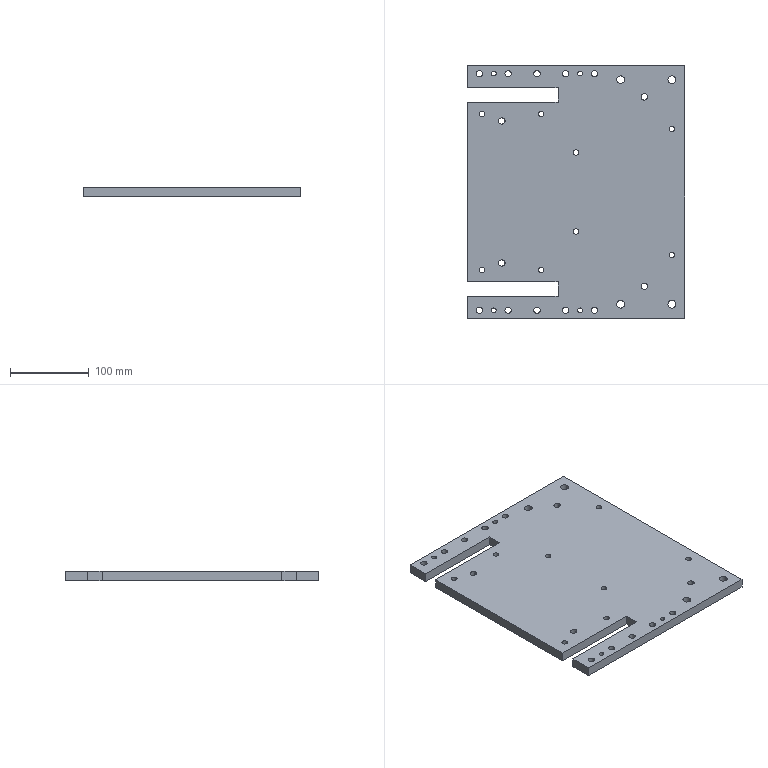Part | STEP file | 1 solid | 87 faces | box 275 x 320 x 12 mm | volume 986186 mm3 | cylinder 62 | plane 22 | cone 3 | commonest cylinder face diameters 1 x24 8 x10 7 x8 6.01 x4 8.01 x4 10 x4